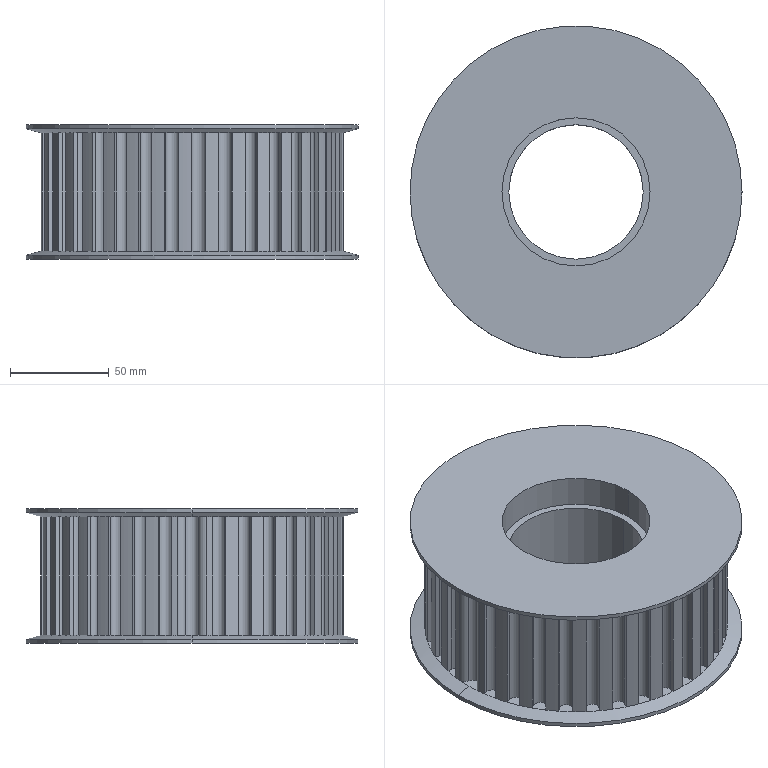Part | STEP file | LM-05-1157 modified_default | 1 solid | 228 faces | box 168 x 168 x 68 mm | volume 926105 mm3 | spline 218 | cylinder 8 | plane 2 | commonest cylinder face diameters 75 x4 7 x2 68 x2